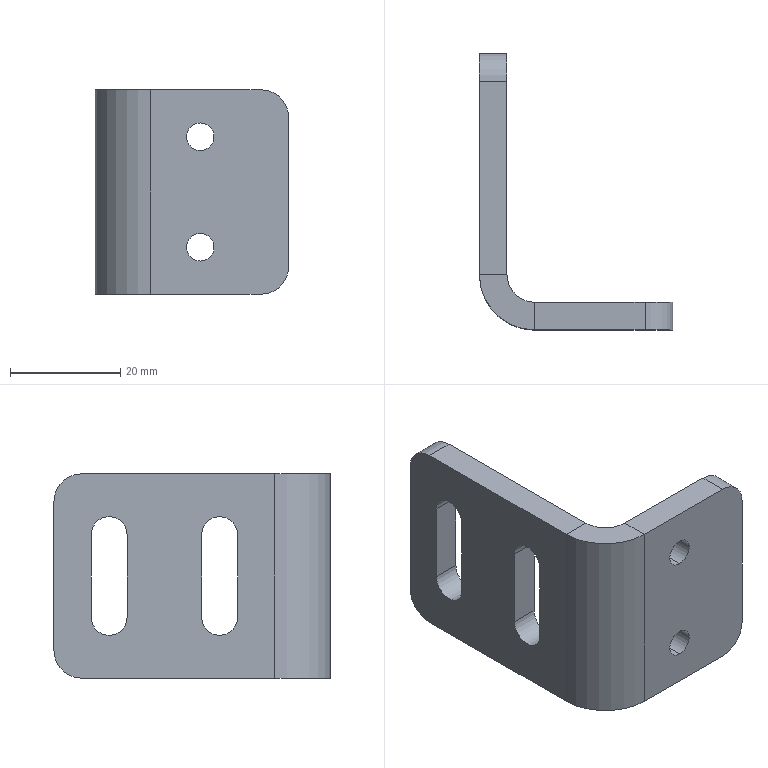Part | SolidWorks | features EdgeFlange 1, Fillet 1, FlatPattern 1, HoleWzd 1, ICE 1, SMBaseFlange 1, SheetMetal 1 | 1 solid | 30 faces | box 35 x 50 x 37 mm | volume 12594 mm3 | plane 16 | cylinder 14 | commonest cylinder face diameters 10 x5 5 x4 6.5 x4 20 x1
STEP:
#1=CARTESIAN_POINT('',(1.5,-5.,-12.5));
#2=VERTEX_POINT('',#1);
#3=CARTESIAN_POINT('',(1.5,-5.,-7.5));
#4=VERTEX_POINT('',#3);
#5=CARTESIAN_POINT('',(1.5,-5.,-10.));
#6=DIRECTION('',(0.,1.,0.));
#7=DIRECTION('',(0.,0.,1.));
#8=AXIS2_PLACEMENT_3D('',#5,#6,#7);
#9=CIRCLE('',#8,2.5);
#10=EDGE_CURVE('',#2,#4,#9,.T.);
#11=ORIENTED_EDGE('',*,*,#10,.F.);
#12=CARTESIAN_POINT('',(1.5,0.,-12.5));
#13=VERTEX_POINT('',#12);
#14=CARTESIAN_POINT('',(1.5,0.,-12.5));
#15=DIRECTION('',(0.,1.,0.));
#16=VECTOR('',#15,1000.);
#17=LINE('',#14,#16);
#18=EDGE_CURVE('',#2,#13,#17,.T.);
#19=ORIENTED_EDGE('',*,*,#18,.T.);
#20=CARTESIAN_POINT('',(1.5,0.,-7.5));
#21=VERTEX_POINT('',#20);
#22=CARTESIAN_POINT('',(1.5,0.,-10.));
#23=DIRECTION('',(0.,1.,0.));
#24=DIRECTION('',(0.,0.,1.));
#25=AXIS2_PLACEMENT_3D('',#22,#23,#24);
#26=CIRCLE('',#25,2.5);
#27=EDGE_CURVE('',#13,#21,#26,.T.);
#28=ORIENTED_EDGE('',*,*,#27,.T.);
#29=CARTESIAN_POINT('',(1.5,0.,-7.5));
#30=DIRECTION('',(0.,1.,0.));
#31=VECTOR('',#30,1000.);
#32=LINE('',#29,#31);
#33=EDGE_CURVE('',#4,#21,#32,.T.);
#34=ORIENTED_EDGE('',*,*,#33,.F.);
#35=EDGE_LOOP('',(#11,#19,#28,#34));
#36=FACE_OUTER_BOUND('',#35,.T.);
#37=CARTESIAN_POINT('',(1.5,0.,-10.));
#38=DIRECTION('',(0.,1.,0.));
#39=DIRECTION('',(0.,0.,1.));
#40=AXIS2_PLACEMENT_3D('',#37,#38,#39);
#41=CYLINDRICAL_SURFACE('',#40,2.5);
#42=ADVANCED_FACE('',(#36),#41,.F.);
#43=CARTESIAN_POINT('',(1.5,-5.,7.5));
#44=VERTEX_POINT('',#43);
#45=CARTESIAN_POINT('',(1.5,-5.,12.5));
#46=VERTEX_POINT('',#45);
#47=CARTESIAN_POINT('',(1.5,-5.,10.));
#48=DIRECTION('',(0.,1.,0.));
#49=DIRECTION('',(0.,0.,1.));
#50=AXIS2_PLACEMENT_3D('',#47,#48,#49);
#51=CIRCLE('',#50,2.5);
#52=EDGE_CURVE('',#44,#46,#51,.T.);
#53=ORIENTED_EDGE('',*,*,#52,.F.);
#54=CARTESIAN_POINT('',(1.5,0.,7.5));
#55=VERTEX_POINT('',#54);
#56=CARTESIAN_POINT('',(1.5,0.,7.5));
#57=DIRECTION('',(0.,1.,0.));
#58=VECTOR('',#57,1000.);
#59=LINE('',#56,#58);
#60=EDGE_CURVE('',#44,#55,#59,.T.);
#61=ORIENTED_EDGE('',*,*,#60,.T.);
#62=CARTESIAN_POINT('',(1.5,0.,12.5));
#63=VERTEX_POINT('',#62);
#64=CARTESIAN_POINT('',(1.5,0.,10.));
#65=DIRECTION('',(0.,1.,0.));
#66=DIRECTION('',(0.,0.,1.));
#67=AXIS2_PLACEMENT_3D('',#64,#65,#66);
#68=CIRCLE('',#67,2.5);
#69=EDGE_CURVE('',#55,#63,#68,.T.);
#70=ORIENTED_EDGE('',*,*,#69,.T.);
#71=CARTESIAN_POINT('',(1.5,0.,12.5));
#72=DIRECTION('',(0.,1.,0.));
#73=VECTOR('',#72,1000.);
#74=LINE('',#71,#73);
#75=EDGE_CURVE('',#46,#63,#74,.T.);
#76=ORIENTED_EDGE('',*,*,#75,.F.);
#77=EDGE_LOOP('',(#53,#61,#70,#76));
#78=FACE_OUTER_BOUND('',#77,.T.);
#79=CARTESIAN_POINT('',(1.5,0.,10.));
#80=DIRECTION('',(0.,1.,0.));
#81=DIRECTION('',(0.,0.,1.));
#82=AXIS2_PLACEMENT_3D('',#79,#80,#81);
#83=CYLINDRICAL_SURFACE('',#82,2.5);
#84=ADVANCED_FACE('',(#78),#83,.F.);
#85=CARTESIAN_POINT('',(-7.5,-5.,18.5));
#86=VERTEX_POINT('',#85);
#87=CARTESIAN_POINT('',(12.5,-5.,18.5));
#88=VERTEX_POINT('',#87);
#89=CARTESIAN_POINT('',(17.5,-5.,18.5));
#90=DIRECTION('',(1.,0.,0.));
#91=VECTOR('',#90,1000.);
#92=LINE('',#89,#91);
#93=EDGE_CURVE('',#86,#88,#92,.T.);
#94=ORIENTED_EDGE('',*,*,#93,.T.);
#95=CARTESIAN_POINT('',(12.5,0.,18.5));
#96=VERTEX_POINT('',#95);
#97=CARTESIAN_POINT('',(12.5,-5.,18.5));
#98=DIRECTION('',(0.,1.,0.));
#99=VECTOR('',#98,1000.);
#100=LINE('',#97,#99);
#101=EDGE_CURVE('',#88,#96,#100,.T.);
#102=ORIENTED_EDGE('',*,*,#101,.T.);
#103=CARTESIAN_POINT('',(-7.5,0.,18.5));
#104=VERTEX_POINT('',#103);
#105=CARTESIAN_POINT('',(17.5,0.,18.5));
#106=DIRECTION('',(1.,0.,0.));
#107=VECTOR('',#106,1000.);
#108=LINE('',#105,#107);
#109=EDGE_CURVE('',#104,#96,#108,.T.);
#110=ORIENTED_EDGE('',*,*,#109,.F.);
#111=CARTESIAN_POINT('',(-7.5,0.,18.5));
#112=DIRECTION('',(0.,-1.,0.));
#113=VECTOR('',#112,1000.);
#114=LINE('',#111,#113);
#115=EDGE_CURVE('',#104,#86,#114,.T.);
#116=ORIENTED_EDGE('',*,*,#115,.T.);
#117=EDGE_LOOP('',(#94,#102,#110,#116));
#118=FACE_OUTER_BOUND('',#117,.T.);
#119=CARTESIAN_POINT('',(17.5,-5.,18.5));
#120=DIRECTION('',(0.,0.,1.));
#121=DIRECTION('',(1.,0.,0.));
#122=AXIS2_PLACEMENT_3D('',#119,#120,#121);
#123=PLANE('',#122);
#124=ADVANCED_FACE('',(#118),#123,.T.);
#125=CARTESIAN_POINT('',(1.5,-5.,10.));
#126=DIRECTION('',(0.,1.,0.));
#127=DIRECTION('',(0.,0.,1.));
#128=AXIS2_PLACEMENT_3D('',#125,#126,#127);
#129=CIRCLE('',#128,2.5);
#130=EDGE_CURVE('',#46,#44,#129,.T.);
#131=ORIENTED_EDGE('',*,*,#130,.T.);
#132=ORIENTED_EDGE('',*,*,#52,.T.);
#133=EDGE_LOOP('',(#131,#132));
#134=FACE_BOUND('',#133,.T.);
#135=CARTESIAN_POINT('',(1.5,-5.,-10.));
#136=DIRECTION('',(0.,1.,0.));
#137=DIRECTION('',(0.,0.,1.));
#138=AXIS2_PLACEMENT_3D('',#135,#136,#137);
#139=CIRCLE('',#138,2.5);
#140=EDGE_CURVE('',#4,#2,#139,.T.);
#141=ORIENTED_EDGE('',*,*,#140,.T.);
#142=ORIENTED_EDGE('',*,*,#10,.T.);
#143=EDGE_LOOP('',(#141,#142));
#144=FACE_BOUND('',#143,.T.);
#145=CARTESIAN_POINT('',(17.5,-5.,13.5));
#146=VERTEX_POINT('',#145);
#147=CARTESIAN_POINT('',(17.5,-5.,-13.5));
#148=VERTEX_POINT('',#147);
#149=CARTESIAN_POINT('',(17.5,-5.,18.5));
#150=DIRECTION('',(0.,0.,-1.));
#151=VECTOR('',#150,1000.);
#152=LINE('',#149,#151);
#153=EDGE_CURVE('',#146,#148,#152,.T.);
#154=ORIENTED_EDGE('',*,*,#153,.F.);
#155=CARTESIAN_POINT('',(12.5,-5.,13.5));
#156=DIRECTION('',(0.,-1.,0.));
#157=DIRECTION('',(0.,0.,1.));
#158=AXIS2_PLACEMENT_3D('',#155,#156,#157);
#159=CIRCLE('',#158,5.);
#160=EDGE_CURVE('',#146,#88,#159,.T.);
#161=ORIENTED_EDGE('',*,*,#160,.T.);
#162=ORIENTED_EDGE('',*,*,#93,.F.);
#163=CARTESIAN_POINT('',(-7.5,-5.,-18.5));
#164=VERTEX_POINT('',#163);
#165=CARTESIAN_POINT('',(-7.5,-5.,18.5));
#166=DIRECTION('',(0.,0.,-1.));
#167=VECTOR('',#166,1000.);
#168=LINE('',#165,#167);
#169=EDGE_CURVE('',#86,#164,#168,.T.);
#170=ORIENTED_EDGE('',*,*,#169,.T.);
#171=CARTESIAN_POINT('',(12.5,-5.,-18.5));
#172=VERTEX_POINT('',#171);
#173=CARTESIAN_POINT('',(17.5,-5.,-18.5));
#174=DIRECTION('',(-1.,0.,0.));
#175=VECTOR('',#174,1000.);
#176=LINE('',#173,#175);
#177=EDGE_CURVE('',#172,#164,#176,.T.);
#178=ORIENTED_EDGE('',*,*,#177,.F.);
#179=CARTESIAN_POINT('',(12.5,-5.,-13.5));
#180=DIRECTION('',(0.,-1.,0.));
#181=DIRECTION('',(0.,0.,1.));
#182=AXIS2_PLACEMENT_3D('',#179,#180,#181);
#183=CIRCLE('',#182,5.);
#184=EDGE_CURVE('',#172,#148,#183,.T.);
#185=ORIENTED_EDGE('',*,*,#184,.T.);
#186=EDGE_LOOP('',(#154,#161,#162,#170,#178,#185));
#187=FACE_OUTER_BOUND('',#186,.T.);
#188=CARTESIAN_POINT('',(0.,-5.,0.));
#189=DIRECTION('',(0.,1.,0.));
#190=DIRECTION('',(0.,0.,1.));
#191=AXIS2_PLACEMENT_3D('',#188,#189,#190);
#192=PLANE('',#191);
#193=ADVANCED_FACE('',(#134,#144,#187),#192,.F.);
#194=CARTESIAN_POINT('',(1.5,0.,-10.));
#195=DIRECTION('',(0.,1.,0.));
#196=DIRECTION('',(0.,0.,1.));
#197=AXIS2_PLACEMENT_3D('',#194,#195,#196);
#198=CIRCLE('',#197,2.5);
#199=EDGE_CURVE('',#21,#13,#198,.T.);
#200=ORIENTED_EDGE('',*,*,#199,.F.);
#201=ORIENTED_EDGE('',*,*,#27,.F.);
#202=EDGE_LOOP('',(#200,#201));
#203=FACE_BOUND('',#202,.T.);
#204=CARTESIAN_POINT('',(1.5,0.,10.));
#205=DIRECTION('',(0.,1.,0.));
#206=DIRECTION('',(0.,0.,1.));
#207=AXIS2_PLACEMENT_3D('',#204,#205,#206);
#208=CIRCLE('',#207,2.5);
#209=EDGE_CURVE('',#63,#55,#208,.T.);
#210=ORIENTED_EDGE('',*,*,#209,.F.);
#211=ORIENTED_EDGE('',*,*,#69,.F.);
#212=EDGE_LOOP('',(#210,#211));
#213=FACE_BOUND('',#212,.T.);
#214=ORIENTED_EDGE('',*,*,#109,.T.);
#215=CARTESIAN_POINT('',(17.5,0.,13.5));
#216=VERTEX_POINT('',#215);
#217=CARTESIAN_POINT('',(12.5,0.,13.5));
#218=DIRECTION('',(0.,1.,0.));
#219=DIRECTION('',(0.,0.,1.));
#220=AXIS2_PLACEMENT_3D('',#217,#218,#219);
#221=CIRCLE('',#220,5.);
#222=EDGE_CURVE('',#96,#216,#221,.T.);
#223=ORIENTED_EDGE('',*,*,#222,.T.);
#224=CARTESIAN_POINT('',(17.5,0.,-13.5));
#225=VERTEX_POINT('',#224);
#226=CARTESIAN_POINT('',(17.5,0.,18.5));
#227=DIRECTION('',(0.,0.,-1.));
#228=VECTOR('',#227,1000.);
#229=LINE('',#226,#228);
#230=EDGE_CURVE('',#216,#225,#229,.T.);
#231=ORIENTED_EDGE('',*,*,#230,.T.);
#232=CARTESIAN_POINT('',(12.5,0.,-18.5));
#233=VERTEX_POINT('',#232);
#234=CARTESIAN_POINT('',(12.5,0.,-13.5));
#235=DIRECTION('',(0.,1.,0.));
#236=DIRECTION('',(0.,0.,1.));
#237=AXIS2_PLACEMENT_3D('',#234,#235,#236);
#238=CIRCLE('',#237,5.);
#239=EDGE_CURVE('',#225,#233,#238,.T.);
#240=ORIENTED_EDGE('',*,*,#239,.T.);
#241=CARTESIAN_POINT('',(-7.5,0.,-18.5));
#242=VERTEX_POINT('',#241);
#243=CARTESIAN_POINT('',(17.5,0.,-18.5));
#244=DIRECTION('',(-1.,0.,0.));
#245=VECTOR('',#244,1000.);
#246=LINE('',#243,#245);
#247=EDGE_CURVE('',#233,#242,#246,.T.);
#248=ORIENTED_EDGE('',*,*,#247,.T.);
#249=CARTESIAN_POINT('',(-7.5,0.,18.5));
#250=DIRECTION('',(0.,0.,-1.));
#251=VECTOR('',#250,1000.);
#252=LINE('',#249,#251);
#253=EDGE_CURVE('',#104,#242,#252,.T.);
#254=ORIENTED_EDGE('',*,*,#253,.F.);
#255=EDGE_LOOP('',(#214,#223,#231,#240,#248,#254));
#256=FACE_OUTER_BOUND('',#255,.T.);
#257=CARTESIAN_POINT('',(0.,0.,0.));
#258=DIRECTION('',(0.,1.,0.));
#259=DIRECTION('',(0.,0.,1.));
#260=AXIS2_PLACEMENT_3D('',#257,#258,#259);
#261=PLANE('',#260);
#262=ADVANCED_FACE('',(#203,#213,#256),#261,.T.);
#263=ORIENTED_EDGE('',*,*,#247,.F.);
#264=CARTESIAN_POINT('',(12.5,-5.,-18.5));
#265=DIRECTION('',(0.,-1.,0.));
#266=VECTOR('',#265,1000.);
#267=LINE('',#264,#266);
#268=EDGE_CURVE('',#233,#172,#267,.T.);
#269=ORIENTED_EDGE('',*,*,#268,.T.);
#270=ORIENTED_EDGE('',*,*,#177,.T.);
#271=CARTESIAN_POINT('',(-7.5,0.,-18.5));
#272=DIRECTION('',(0.,-1.,0.));
#273=VECTOR('',#272,1000.);
#274=LINE('',#271,#273);
#275=EDGE_CURVE('',#242,#164,#274,.T.);
#276=ORIENTED_EDGE('',*,*,#275,.F.);
#277=EDGE_LOOP('',(#263,#269,#270,#276));
#278=FACE_OUTER_BOUND('',#277,.T.);
#279=CARTESIAN_POINT('',(17.5,-5.,-18.5));
#280=DIRECTION('',(0.,0.,-1.));
#281=DIRECTION('',(-1.,0.,0.));
#282=AXIS2_PLACEMENT_3D('',#279,#280,#281);
#283=PLANE('',#282);
#284=ADVANCED_FACE('',(#278),#283,.T.);
#285=ORIENTED_EDGE('',*,*,#230,.F.);
#286=CARTESIAN_POINT('',(17.5,-5.,13.5));
#287=DIRECTION('',(0.,-1.,0.));
#288=VECTOR('',#287,1000.);
#289=LINE('',#286,#288);
#290=EDGE_CURVE('',#216,#146,#289,.T.);
#291=ORIENTED_EDGE('',*,*,#290,.T.);
#292=ORIENTED_EDGE('',*,*,#153,.T.);
#293=CARTESIAN_POINT('',(17.5,-5.,-13.5));
#294=DIRECTION('',(0.,1.,0.));
#295=VECTOR('',#294,1000.);
#296=LINE('',#293,#295);
#297=EDGE_CURVE('',#148,#225,#296,.T.);
#298=ORIENTED_EDGE('',*,*,#297,.T.);
#299=EDGE_LOOP('',(#285,#291,#292,#298));
#300=FACE_OUTER_BOUND('',#299,.T.);
#301=CARTESIAN_POINT('',(17.5,-5.,18.5));
#302=DIRECTION('',(1.,0.,0.));
#303=DIRECTION('',(0.,0.,-1.));
#304=AXIS2_PLACEMENT_3D('',#301,#302,#303);
#305=PLANE('',#304);
#306=ADVANCED_FACE('',(#300),#305,.T.);
#307=ORIENTED_EDGE('',*,*,#60,.F.);
#308=ORIENTED_EDGE('',*,*,#130,.F.);
#309=ORIENTED_EDGE('',*,*,#75,.T.);
#310=ORIENTED_EDGE('',*,*,#209,.T.);
#311=EDGE_LOOP('',(#307,#308,#309,#310));
#312=FACE_OUTER_BOUND('',#311,.T.);
#313=CARTESIAN_POINT('',(1.5,0.,10.));
#314=DIRECTION('',(0.,1.,0.));
#315=DIRECTION('',(0.,0.,1.));
#316=AXIS2_PLACEMENT_3D('',#313,#314,#315);
#317=CYLINDRICAL_SURFACE('',#316,2.5);
#318=ADVANCED_FACE('',(#312),#317,.F.);
#319=ORIENTED_EDGE('',*,*,#18,.F.);
#320=ORIENTED_EDGE('',*,*,#140,.F.);
#321=ORIENTED_EDGE('',*,*,#33,.T.);
#322=ORIENTED_EDGE('',*,*,#199,.T.);
#323=EDGE_LOOP('',(#319,#320,#321,#322));
#324=FACE_OUTER_BOUND('',#323,.T.);
#325=CARTESIAN_POINT('',(1.5,0.,-10.));
#326=DIRECTION('',(0.,1.,0.));
#327=DIRECTION('',(0.,0.,1.));
#328=AXIS2_PLACEMENT_3D('',#325,#326,#327);
#329=CYLINDRICAL_SURFACE('',#328,2.5);
#330=ADVANCED_FACE('',(#324),#329,.F.);
#331=CARTESIAN_POINT('',(-12.5,5.,-18.5));
#332=VERTEX_POINT('',#331);
#333=CARTESIAN_POINT('',(-17.5,5.,-18.5));
#334=VERTEX_POINT('',#333);
#335=CARTESIAN_POINT('',(-17.5,5.,-18.5));
#336=DIRECTION('',(-1.,0.,0.));
#337=VECTOR('',#336,1000.);
#338=LINE('',#335,#337);
#339=EDGE_CURVE('',#332,#334,#338,.T.);
#340=ORIENTED_EDGE('',*,*,#339,.F.);
#341=CARTESIAN_POINT('',(-7.5,5.,-18.5));
#342=DIRECTION('',(0.,0.,-1.));
#343=DIRECTION('',(0.,-1.,0.));
#344=AXIS2_PLACEMENT_3D('',#341,#342,#343);
#345=CIRCLE('',#344,5.);
#346=EDGE_CURVE('',#242,#332,#345,.T.);
#347=ORIENTED_EDGE('',*,*,#346,.F.);
#348=ORIENTED_EDGE('',*,*,#275,.T.);
#349=CARTESIAN_POINT('',(-7.5,5.,-18.5));
#350=DIRECTION('',(0.,0.,-1.));
#351=DIRECTION('',(0.,-1.,0.));
#352=AXIS2_PLACEMENT_3D('',#349,#350,#351);
#353=CIRCLE('',#352,10.);
#354=EDGE_CURVE('',#164,#334,#353,.T.);
#355=ORIENTED_EDGE('',*,*,#354,.T.);
#356=EDGE_LOOP('',(#340,#347,#348,#355));
#357=FACE_OUTER_BOUND('',#356,.T.);
#358=CARTESIAN_POINT('',(-7.5,5.,-18.5));
#359=DIRECTION('',(0.,0.,-1.));
#360=DIRECTION('',(0.,1.,0.));
#361=AXIS2_PLACEMENT_3D('',#358,#359,#360);
#362=PLANE('',#361);
#363=ADVANCED_FACE('',(#357),#362,.T.);
#364=CARTESIAN_POINT('',(-12.5,5.,18.5));
#365=VERTEX_POINT('',#364);
#366=CARTESIAN_POINT('',(-7.5,5.,18.5));
#367=DIRECTION('',(0.,0.,1.));
#368=DIRECTION('',(0.,-1.,0.));
#369=AXIS2_PLACEMENT_3D('',#366,#367,#368);
#370=CIRCLE('',#369,5.);
#371=EDGE_CURVE('',#365,#104,#370,.T.);
#372=ORIENTED_EDGE('',*,*,#371,.F.);
#373=CARTESIAN_POINT('',(-17.5,5.,18.5));
#374=VERTEX_POINT('',#373);
#375=CARTESIAN_POINT('',(-12.5,5.,18.5));
#376=DIRECTION('',(-1.,0.,0.));
#377=VECTOR('',#376,1000.);
#378=LINE('',#375,#377);
#379=EDGE_CURVE('',#365,#374,#378,.T.);
#380=ORIENTED_EDGE('',*,*,#379,.T.);
#381=CARTESIAN_POINT('',(-7.5,5.,18.5));
#382=DIRECTION('',(0.,0.,1.));
#383=DIRECTION('',(0.,-1.,0.));
#384=AXIS2_PLACEMENT_3D('',#381,#382,#383);
#385=CIRCLE('',#384,10.);
#386=EDGE_CURVE('',#374,#86,#385,.T.);
#387=ORIENTED_EDGE('',*,*,#386,.T.);
#388=ORIENTED_EDGE('',*,*,#115,.F.);
#389=EDGE_LOOP('',(#372,#380,#387,#388));
#390=FACE_OUTER_BOUND('',#389,.T.);
#391=CARTESIAN_POINT('',(-7.5,5.,18.5));
#392=DIRECTION('',(0.,0.,-1.));
#393=DIRECTION('',(0.,1.,0.));
#394=AXIS2_PLACEMENT_3D('',#391,#392,#393);
#395=PLANE('',#394);
#396=ADVANCED_FACE('',(#390),#395,.F.);
#397=ORIENTED_EDGE('',*,*,#169,.F.);
#398=ORIENTED_EDGE('',*,*,#386,.F.);
#399=CARTESIAN_POINT('',(-17.5,5.,-18.5));
#400=DIRECTION('',(0.,0.,-1.));
#401=VECTOR('',#400,1000.);
#402=LINE('',#399,#401);
#403=EDGE_CURVE('',#374,#334,#402,.T.);
#404=ORIENTED_EDGE('',*,*,#403,.T.);
#405=ORIENTED_EDGE('',*,*,#354,.F.);
#406=EDGE_LOOP('',(#397,#398,#404,#405));
#407=FACE_OUTER_BOUND('',#406,.T.);
#408=CARTESIAN_POINT('',(-7.5,5.,18.5));
#409=DIRECTION('',(0.,0.,1.));
#410=DIRECTION('',(-1.,0.,0.));
#411=AXIS2_PLACEMENT_3D('',#408,#409,#410);
#412=CYLINDRICAL_SURFACE('',#411,10.);
#413=ADVANCED_FACE('',(#407),#412,.T.);
#414=ORIENTED_EDGE('',*,*,#253,.T.);
#415=ORIENTED_EDGE('',*,*,#346,.T.);
#416=CARTESIAN_POINT('',(-12.5,5.,-18.5));
#417=DIRECTION('',(0.,0.,1.));
#418=VECTOR('',#417,1000.);
#419=LINE('',#416,#418);
#420=EDGE_CURVE('',#332,#365,#419,.T.);
#421=ORIENTED_EDGE('',*,*,#420,.T.);
#422=ORIENTED_EDGE('',*,*,#371,.T.);
#423=EDGE_LOOP('',(#414,#415,#421,#422));
#424=FACE_OUTER_BOUND('',#423,.T.);
#425=CARTESIAN_POINT('',(-7.5,5.,18.5));
#426=DIRECTION('',(0.,0.,1.));
#427=DIRECTION('',(-1.,0.,0.));
#428=AXIS2_PLACEMENT_3D('',#425,#426,#427);
#429=CYLINDRICAL_SURFACE('',#428,5.);
#430=ADVANCED_FACE('',(#424),#429,.F.);
#431=CARTESIAN_POINT('',(-17.5,40.,-18.5));
#432=VERTEX_POINT('',#431);
#433=CARTESIAN_POINT('',(-17.5,0.,-18.5));
#434=DIRECTION('',(0.,-1.,0.));
#435=VECTOR('',#434,1000.);
#436=LINE('',#433,#435);
#437=EDGE_CURVE('',#432,#334,#436,.T.);
#438=ORIENTED_EDGE('',*,*,#437,.F.);
#439=CARTESIAN_POINT('',(-12.5,40.,-18.5));
#440=VERTEX_POINT('',#439);
#441=CARTESIAN_POINT('',(-17.5,40.,-18.5));
#442=DIRECTION('',(1.,0.,0.));
#443=VECTOR('',#442,1000.);
#444=LINE('',#441,#443);
#445=EDGE_CURVE('',#432,#440,#444,.T.);
#446=ORIENTED_EDGE('',*,*,#445,.T.);
#447=CARTESIAN_POINT('',(-12.5,0.,-18.5));
#448=DIRECTION('',(0.,-1.,0.));
#449=VECTOR('',#448,1000.);
#450=LINE('',#447,#449);
#451=EDGE_CURVE('',#440,#332,#450,.T.);
#452=ORIENTED_EDGE('',*,*,#451,.T.);
#453=ORIENTED_EDGE('',*,*,#339,.T.);
#454=EDGE_LOOP('',(#438,#446,#452,#453));
#455=FACE_OUTER_BOUND('',#454,.T.);
#456=CARTESIAN_POINT('',(-17.5,0.,-18.5));
#457=DIRECTION('',(0.,0.,1.));
#458=DIRECTION('',(1.,0.,0.));
#459=AXIS2_PLACEMENT_3D('',#456,#457,#458);
#460=PLANE('',#459);
#461=ADVANCED_FACE('',(#455),#460,.F.);
#462=CARTESIAN_POINT('',(-12.5,40.,18.5));
#463=VERTEX_POINT('',#462);
#464=CARTESIAN_POINT('',(-12.5,45.,18.5));
#465=DIRECTION('',(0.,1.,0.));
#466=VECTOR('',#465,1000.);
#467=LINE('',#464,#466);
#468=EDGE_CURVE('',#365,#463,#467,.T.);
#469=ORIENTED_EDGE('',*,*,#468,.T.);
#470=CARTESIAN_POINT('',(-17.5,40.,18.5));
#471=VERTEX_POINT('',#470);
#472=CARTESIAN_POINT('',(-17.5,40.,18.5));
#473=DIRECTION('',(-1.,0.,0.));
#474=VECTOR('',#473,1000.);
#475=LINE('',#472,#474);
#476=EDGE_CURVE('',#463,#471,#475,.T.);
#477=ORIENTED_EDGE('',*,*,#476,.T.);
#478=CARTESIAN_POINT('',(-17.5,0.,18.5));
#479=DIRECTION('',(0.,1.,0.));
#480=VECTOR('',#479,1000.);
#481=LINE('',#478,#480);
#482=EDGE_CURVE('',#374,#471,#481,.T.);
#483=ORIENTED_EDGE('',*,*,#482,.F.);
#484=ORIENTED_EDGE('',*,*,#379,.F.);
#485=EDGE_LOOP('',(#469,#477,#483,#484));
#486=FACE_OUTER_BOUND('',#485,.T.);
#487=CARTESIAN_POINT('',(-17.5,45.,18.5));
#488=DIRECTION('',(0.,0.,-1.));
#489=DIRECTION('',(-1.,0.,0.));
#490=AXIS2_PLACEMENT_3D('',#487,#488,#489);
#491=PLANE('',#490);
#492=ADVANCED_FACE('',(#486),#491,.F.);
#493=CARTESIAN_POINT('',(-17.5,31.75,7.5));
#494=VERTEX_POINT('',#493);
#495=CARTESIAN_POINT('',(-17.5,31.75,-7.5));
#496=VERTEX_POINT('',#495);
#497=CARTESIAN_POINT('',(-17.5,31.75,0.));
#498=DIRECTION('',(0.,0.,-1.));
#499=VECTOR('',#498,1000.);
#500=LINE('',#497,#499);
#501=EDGE_CURVE('',#494,#496,#500,.T.);
#502=ORIENTED_EDGE('',*,*,#501,.T.);
#503=CARTESIAN_POINT('',(-17.5,38.25,-7.5));
#504=VERTEX_POINT('',#503);
#505=CARTESIAN_POINT('',(-17.5,35.,-7.5));
#506=DIRECTION('',(1.,0.,0.));
#507=DIRECTION('',(0.,1.,0.));
#508=AXIS2_PLACEMENT_3D('',#505,#506,#507);
#509=CIRCLE('',#508,3.25);
#510=EDGE_CURVE('',#496,#504,#509,.T.);
#511=ORIENTED_EDGE('',*,*,#510,.T.);
#512=CARTESIAN_POINT('',(-17.5,38.25,7.5));
#513=VERTEX_POINT('',#512);
#514=CARTESIAN_POINT('',(-17.5,38.25,0.));
#515=DIRECTION('',(0.,0.,1.));
#516=VECTOR('',#515,1000.);
#517=LINE('',#514,#516);
#518=EDGE_CURVE('',#504,#513,#517,.T.);
#519=ORIENTED_EDGE('',*,*,#518,.T.);
#520=CARTESIAN_POINT('',(-17.5,35.,7.5));
#521=DIRECTION('',(1.,0.,0.));
#522=DIRECTION('',(0.,1.,0.));
#523=AXIS2_PLACEMENT_3D('',#520,#521,#522);
#524=CIRCLE('',#523,3.25);
#525=EDGE_CURVE('',#513,#494,#524,.T.);
#526=ORIENTED_EDGE('',*,*,#525,.T.);
#527=EDGE_LOOP('',(#502,#511,#519,#526));
#528=FACE_BOUND('',#527,.T.);
#529=CARTESIAN_POINT('',(-17.5,11.75,7.5));
#530=VERTEX_POINT('',#529);
#531=CARTESIAN_POINT('',(-17.5,11.75,-7.5));
#532=VERTEX_POINT('',#531);
#533=CARTESIAN_POINT('',(-17.5,11.75,0.));
#534=DIRECTION('',(0.,0.,-1.));
#535=VECTOR('',#534,1000.);
#536=LINE('',#533,#535);
#537=EDGE_CURVE('',#530,#532,#536,.T.);
#538=ORIENTED_EDGE('',*,*,#537,.T.);
#539=CARTESIAN_POINT('',(-17.5,18.25,-7.5));
#540=VERTEX_POINT('',#539);
#541=CARTESIAN_POINT('',(-17.5,15.,-7.5));
#542=DIRECTION('',(1.,0.,0.));
#543=DIRECTION('',(0.,1.,0.));
#544=AXIS2_PLACEMENT_3D('',#541,#542,#543);
#545=CIRCLE('',#544,3.25);
#546=EDGE_CURVE('',#532,#540,#545,.T.);
#547=ORIENTED_EDGE('',*,*,#546,.T.);
#548=CARTESIAN_POINT('',(-17.5,18.25,7.5));
#549=VERTEX_POINT('',#548);
#550=CARTESIAN_POINT('',(-17.5,18.25,0.));
#551=DIRECTION('',(0.,0.,1.));
#552=VECTOR('',#551,1000.);
#553=LINE('',#550,#552);
#554=EDGE_CURVE('',#540,#549,#553,.T.);
#555=ORIENTED_EDGE('',*,*,#554,.T.);
#556=CARTESIAN_POINT('',(-17.5,15.,7.5));
#557=DIRECTION('',(1.,0.,0.));
#558=DIRECTION('',(0.,1.,0.));
#559=AXIS2_PLACEMENT_3D('',#556,#557,#558);
#560=CIRCLE('',#559,3.25);
#561=EDGE_CURVE('',#549,#530,#560,.T.);
#562=ORIENTED_EDGE('',*,*,#561,.T.);
#563=EDGE_LOOP('',(#538,#547,#555,#562));
#564=FACE_BOUND('',#563,.T.);
#565=CARTESIAN_POINT('',(-17.5,45.,13.5));
#566=VERTEX_POINT('',#565);
#567=CARTESIAN_POINT('',(-17.5,45.,-13.5));
#568=VERTEX_POINT('',#567);
#569=CARTESIAN_POINT('',(-17.5,45.,0.));
#570=DIRECTION('',(0.,0.,-1.));
#571=VECTOR('',#570,1000.);
#572=LINE('',#569,#571);
#573=EDGE_CURVE('',#566,#568,#572,.T.);
#574=ORIENTED_EDGE('',*,*,#573,.T.);
#575=CARTESIAN_POINT('',(-17.5,40.,-13.5));
#576=DIRECTION('',(-1.,0.,0.));
#577=DIRECTION('',(0.,1.,0.));
#578=AXIS2_PLACEMENT_3D('',#575,#576,#577);
#579=CIRCLE('',#578,5.);
#580=EDGE_CURVE('',#568,#432,#579,.T.);
#581=ORIENTED_EDGE('',*,*,#580,.T.);
#582=ORIENTED_EDGE('',*,*,#437,.T.);
#583=ORIENTED_EDGE('',*,*,#403,.F.);
#584=ORIENTED_EDGE('',*,*,#482,.T.);
#585=CARTESIAN_POINT('',(-17.5,40.,13.5));
#586=DIRECTION('',(-1.,0.,0.));
#587=DIRECTION('',(0.,1.,0.));
#588=AXIS2_PLACEMENT_3D('',#585,#586,#587);
#589=CIRCLE('',#588,5.);
#590=EDGE_CURVE('',#471,#566,#589,.T.);
#591=ORIENTED_EDGE('',*,*,#590,.T.);
#592=EDGE_LOOP('',(#574,#581,#582,#583,#584,#591));
#593=FACE_OUTER_BOUND('',#592,.T.);
#594=CARTESIAN_POINT('',(-17.5,0.,0.));
#595=DIRECTION('',(1.,0.,0.));
#596=DIRECTION('',(0.,1.,0.));
#597=AXIS2_PLACEMENT_3D('',#594,#595,#596);
#598=PLANE('',#597);
#599=ADVANCED_FACE('',(#528,#564,#593),#598,.F.);
#600=CARTESIAN_POINT('',(-12.5,31.75,-7.5));
#601=VERTEX_POINT('',#600);
#602=CARTESIAN_POINT('',(-12.5,38.25,-7.5));
#603=VERTEX_POINT('',#602);
#604=CARTESIAN_POINT('',(-12.5,35.,-7.5));
#605=DIRECTION('',(1.,0.,0.));
#606=DIRECTION('',(0.,1.,0.));
#607=AXIS2_PLACEMENT_3D('',#604,#605,#606);
#608=CIRCLE('',#607,3.25);
#609=EDGE_CURVE('',#601,#603,#608,.T.);
#610=ORIENTED_EDGE('',*,*,#609,.F.);
#611=CARTESIAN_POINT('',(-12.5,31.75,7.5));
#612=VERTEX_POINT('',#611);
#613=CARTESIAN_POINT('',(-12.5,31.75,-7.5));
#614=DIRECTION('',(0.,0.,-1.));
#615=VECTOR('',#614,1000.);
#616=LINE('',#613,#615);
#617=EDGE_CURVE('',#612,#601,#616,.T.);
#618=ORIENTED_EDGE('',*,*,#617,.F.);
#619=CARTESIAN_POINT('',(-12.5,38.25,7.5));
#620=VERTEX_POINT('',#619);
#621=CARTESIAN_POINT('',(-12.5,35.,7.5));
#622=DIRECTION('',(1.,0.,0.));
#623=DIRECTION('',(0.,1.,0.));
#624=AXIS2_PLACEMENT_3D('',#621,#622,#623);
#625=CIRCLE('',#624,3.25);
#626=EDGE_CURVE('',#620,#612,#625,.T.);
#627=ORIENTED_EDGE('',*,*,#626,.F.);
#628=CARTESIAN_POINT('',(-12.5,38.25,-7.5));
#629=DIRECTION('',(0.,0.,1.));
#630=VECTOR('',#629,1000.);
#631=LINE('',#628,#630);
#632=EDGE_CURVE('',#603,#620,#631,.T.);
#633=ORIENTED_EDGE('',*,*,#632,.F.);
#634=EDGE_LOOP('',(#610,#618,#627,#633));
#635=FACE_BOUND('',#634,.T.);
#636=CARTESIAN_POINT('',(-12.5,11.75,-7.5));
#637=VERTEX_POINT('',#636);
#638=CARTESIAN_POINT('',(-12.5,18.25,-7.5));
#639=VERTEX_POINT('',#638);
#640=CARTESIAN_POINT('',(-12.5,15.,-7.5));
#641=DIRECTION('',(1.,0.,0.));
#642=DIRECTION('',(0.,1.,0.));
#643=AXIS2_PLACEMENT_3D('',#640,#641,#642);
#644=CIRCLE('',#643,3.25);
#645=EDGE_CURVE('',#637,#639,#644,.T.);
#646=ORIENTED_EDGE('',*,*,#645,.F.);
#647=CARTESIAN_POINT('',(-12.5,11.75,7.5));
#648=VERTEX_POINT('',#647);
#649=CARTESIAN_POINT('',(-12.5,11.75,-7.5));
#650=DIRECTION('',(0.,0.,-1.));
#651=VECTOR('',#650,1000.);
#652=LINE('',#649,#651);
#653=EDGE_CURVE('',#648,#637,#652,.T.);
#654=ORIENTED_EDGE('',*,*,#653,.F.);
#655=CARTESIAN_POINT('',(-12.5,18.25,7.5));
#656=VERTEX_POINT('',#655);
#657=CARTESIAN_POINT('',(-12.5,15.,7.5));
#658=DIRECTION('',(1.,0.,0.));
#659=DIRECTION('',(0.,1.,0.));
#660=AXIS2_PLACEMENT_3D('',#657,#658,#659);
#661=CIRCLE('',#660,3.25);
#662=EDGE_CURVE('',#656,#648,#661,.T.);
#663=ORIENTED_EDGE('',*,*,#662,.F.);
#664=CARTESIAN_POINT('',(-12.5,18.25,-7.5));
#665=DIRECTION('',(0.,0.,1.));
#666=VECTOR('',#665,1000.);
#667=LINE('',#664,#666);
#668=EDGE_CURVE('',#639,#656,#667,.T.);
#669=ORIENTED_EDGE('',*,*,#668,.F.);
#670=EDGE_LOOP('',(#646,#654,#663,#669));
#671=FACE_BOUND('',#670,.T.);
#672=ORIENTED_EDGE('',*,*,#451,.F.);
#673=CARTESIAN_POINT('',(-12.5,45.,-13.5));
#674=VERTEX_POINT('',#673);
#675=CARTESIAN_POINT('',(-12.5,40.,-13.5));
#676=DIRECTION('',(1.,0.,0.));
#677=DIRECTION('',(0.,1.,0.));
#678=AXIS2_PLACEMENT_3D('',#675,#676,#677);
#679=CIRCLE('',#678,5.);
#680=EDGE_CURVE('',#440,#674,#679,.T.);
#681=ORIENTED_EDGE('',*,*,#680,.T.);
#682=CARTESIAN_POINT('',(-12.5,45.,13.5));
#683=VERTEX_POINT('',#682);
#684=CARTESIAN_POINT('',(-12.5,45.,-18.5));
#685=DIRECTION('',(0.,0.,-1.));
#686=VECTOR('',#685,1000.);
#687=LINE('',#684,#686);
#688=EDGE_CURVE('',#683,#674,#687,.T.);
#689=ORIENTED_EDGE('',*,*,#688,.F.);
#690=CARTESIAN_POINT('',(-12.5,40.,13.5));
#691=DIRECTION('',(1.,0.,0.));
#692=DIRECTION('',(0.,1.,0.));
#693=AXIS2_PLACEMENT_3D('',#690,#691,#692);
#694=CIRCLE('',#693,5.);
#695=EDGE_CURVE('',#683,#463,#694,.T.);
#696=ORIENTED_EDGE('',*,*,#695,.T.);
#697=ORIENTED_EDGE('',*,*,#468,.F.);
#698=ORIENTED_EDGE('',*,*,#420,.F.);
#699=EDGE_LOOP('',(#672,#681,#689,#696,#697,#698));
#700=FACE_OUTER_BOUND('',#699,.T.);
#701=CARTESIAN_POINT('',(-12.5,0.,0.));
#702=DIRECTION('',(1.,0.,0.));
#703=DIRECTION('',(0.,1.,0.));
#704=AXIS2_PLACEMENT_3D('',#701,#702,#703);
#705=PLANE('',#704);
#706=ADVANCED_FACE('',(#635,#671,#700),#705,.T.);
#707=ORIENTED_EDGE('',*,*,#688,.T.);
#708=CARTESIAN_POINT('',(-17.5,45.,-13.5));
#709=DIRECTION('',(-1.,0.,0.));
#710=VECTOR('',#709,1000.);
#711=LINE('',#708,#710);
#712=EDGE_CURVE('',#674,#568,#711,.T.);
#713=ORIENTED_EDGE('',*,*,#712,.T.);
#714=ORIENTED_EDGE('',*,*,#573,.F.);
#715=CARTESIAN_POINT('',(-17.5,45.,13.5));
#716=DIRECTION('',(1.,0.,0.));
#717=VECTOR('',#716,1000.);
#718=LINE('',#715,#717);
#719=EDGE_CURVE('',#566,#683,#718,.T.);
#720=ORIENTED_EDGE('',*,*,#719,.T.);
#721=EDGE_LOOP('',(#707,#713,#714,#720));
#722=FACE_OUTER_BOUND('',#721,.T.);
#723=CARTESIAN_POINT('',(-17.5,45.,-18.5));
#724=DIRECTION('',(0.,-1.,0.));
#725=DIRECTION('',(1.,0.,0.));
#726=AXIS2_PLACEMENT_3D('',#723,#724,#725);
#727=PLANE('',#726);
#728=ADVANCED_FACE('',(#722),#727,.F.);
#729=CARTESIAN_POINT('',(-22.5,11.75,-7.5));
#730=DIRECTION('',(1.,0.,0.));
#731=VECTOR('',#730,1000.);
#732=LINE('',#729,#731);
#733=EDGE_CURVE('',#532,#637,#732,.T.);
#734=ORIENTED_EDGE('',*,*,#733,.T.);
#735=ORIENTED_EDGE('',*,*,#645,.T.);
#736=CARTESIAN_POINT('',(-22.5,18.25,-7.5));
#737=DIRECTION('',(1.,0.,0.));
#738=VECTOR('',#737,1000.);
#739=LINE('',#736,#738);
#740=EDGE_CURVE('',#540,#639,#739,.T.);
#741=ORIENTED_EDGE('',*,*,#740,.F.);
#742=ORIENTED_EDGE('',*,*,#546,.F.);
#743=EDGE_LOOP('',(#734,#735,#741,#742));
#744=FACE_OUTER_BOUND('',#743,.T.);
#745=CARTESIAN_POINT('',(-22.5,15.,-7.5));
#746=DIRECTION('',(1.,0.,0.));
#747=DIRECTION('',(0.,1.,0.));
#748=AXIS2_PLACEMENT_3D('',#745,#746,#747);
#749=CYLINDRICAL_SURFACE('',#748,3.25);
#750=ADVANCED_FACE('',(#744),#749,.F.);
#751=CARTESIAN_POINT('',(-22.5,11.75,7.5));
#752=DIRECTION('',(1.,0.,0.));
#753=VECTOR('',#752,1000.);
#754=LINE('',#751,#753);
#755=EDGE_CURVE('',#530,#648,#754,.T.);
#756=ORIENTED_EDGE('',*,*,#755,.T.);
#757=ORIENTED_EDGE('',*,*,#653,.T.);
#758=ORIENTED_EDGE('',*,*,#733,.F.);
#759=ORIENTED_EDGE('',*,*,#537,.F.);
#760=EDGE_LOOP('',(#756,#757,#758,#759));
#761=FACE_OUTER_BOUND('',#760,.T.);
#762=CARTESIAN_POINT('',(-22.5,11.75,-7.5));
#763=DIRECTION('',(0.,-1.,0.));
#764=DIRECTION('',(1.,0.,0.));
#765=AXIS2_PLACEMENT_3D('',#762,#763,#764);
#766=PLANE('',#765);
#767=ADVANCED_FACE('',(#761),#766,.F.);
#768=CARTESIAN_POINT('',(-22.5,18.25,7.5));
#769=DIRECTION('',(1.,0.,0.));
#770=VECTOR('',#769,1000.);
#771=LINE('',#768,#770);
#772=EDGE_CURVE('',#549,#656,#771,.T.);
#773=ORIENTED_EDGE('',*,*,#772,.T.);
#774=ORIENTED_EDGE('',*,*,#662,.T.);
#775=ORIENTED_EDGE('',*,*,#755,.F.);
#776=ORIENTED_EDGE('',*,*,#561,.F.);
#777=EDGE_LOOP('',(#773,#774,#775,#776));
#778=FACE_OUTER_BOUND('',#777,.T.);
#779=CARTESIAN_POINT('',(-22.5,15.,7.5));
#780=DIRECTION('',(1.,0.,0.));
#781=DIRECTION('',(0.,1.,0.));
#782=AXIS2_PLACEMENT_3D('',#779,#780,#781);
#783=CYLINDRICAL_SURFACE('',#782,3.25);
#784=ADVANCED_FACE('',(#778),#783,.F.);
#785=ORIENTED_EDGE('',*,*,#740,.T.);
#786=ORIENTED_EDGE('',*,*,#668,.T.);
#787=ORIENTED_EDGE('',*,*,#772,.F.);
#788=ORIENTED_EDGE('',*,*,#554,.F.);
#789=EDGE_LOOP('',(#785,#786,#787,#788));
#790=FACE_OUTER_BOUND('',#789,.T.);
#791=CARTESIAN_POINT('',(-22.5,18.25,-7.5));
#792=DIRECTION('',(0.,1.,0.));
#793=DIRECTION('',(-1.,0.,0.));
#794=AXIS2_PLACEMENT_3D('',#791,#792,#793);
#795=PLANE('',#794);
#796=ADVANCED_FACE('',(#790),#795,.F.);
#797=CARTESIAN_POINT('',(-22.5,31.75,-7.5));
#798=DIRECTION('',(1.,0.,0.));
#799=VECTOR('',#798,1000.);
#800=LINE('',#797,#799);
#801=EDGE_CURVE('',#496,#601,#800,.T.);
#802=ORIENTED_EDGE('',*,*,#801,.T.);
#803=ORIENTED_EDGE('',*,*,#609,.T.);
#804=CARTESIAN_POINT('',(-22.5,38.25,-7.5));
#805=DIRECTION('',(1.,0.,0.));
#806=VECTOR('',#805,1000.);
#807=LINE('',#804,#806);
#808=EDGE_CURVE('',#504,#603,#807,.T.);
#809=ORIENTED_EDGE('',*,*,#808,.F.);
#810=ORIENTED_EDGE('',*,*,#510,.F.);
#811=EDGE_LOOP('',(#802,#803,#809,#810));
#812=FACE_OUTER_BOUND('',#811,.T.);
#813=CARTESIAN_POINT('',(-22.5,35.,-7.5));
#814=DIRECTION('',(1.,0.,0.));
#815=DIRECTION('',(0.,1.,0.));
#816=AXIS2_PLACEMENT_3D('',#813,#814,#815);
#817=CYLINDRICAL_SURFACE('',#816,3.25);
#818=ADVANCED_FACE('',(#812),#817,.F.);
#819=CARTESIAN_POINT('',(-22.5,31.75,7.5));
#820=DIRECTION('',(1.,0.,0.));
#821=VECTOR('',#820,1000.);
#822=LINE('',#819,#821);
#823=EDGE_CURVE('',#494,#612,#822,.T.);
#824=ORIENTED_EDGE('',*,*,#823,.T.);
#825=ORIENTED_EDGE('',*,*,#617,.T.);
#826=ORIENTED_EDGE('',*,*,#801,.F.);
#827=ORIENTED_EDGE('',*,*,#501,.F.);
#828=EDGE_LOOP('',(#824,#825,#826,#827));
#829=FACE_OUTER_BOUND('',#828,.T.);
#830=CARTESIAN_POINT('',(-22.5,31.75,-7.5));
#831=DIRECTION('',(0.,-1.,0.));
#832=DIRECTION('',(1.,0.,0.));
#833=AXIS2_PLACEMENT_3D('',#830,#831,#832);
#834=PLANE('',#833);
#835=ADVANCED_FACE('',(#829),#834,.F.);
#836=CARTESIAN_POINT('',(-22.5,38.25,7.5));
#837=DIRECTION('',(1.,0.,0.));
#838=VECTOR('',#837,1000.);
#839=LINE('',#836,#838);
#840=EDGE_CURVE('',#513,#620,#839,.T.);
#841=ORIENTED_EDGE('',*,*,#840,.T.);
#842=ORIENTED_EDGE('',*,*,#626,.T.);
#843=ORIENTED_EDGE('',*,*,#823,.F.);
#844=ORIENTED_EDGE('',*,*,#525,.F.);
#845=EDGE_LOOP('',(#841,#842,#843,#844));
#846=FACE_OUTER_BOUND('',#845,.T.);
#847=CARTESIAN_POINT('',(-22.5,35.,7.5));
#848=DIRECTION('',(1.,0.,0.));
#849=DIRECTION('',(0.,1.,0.));
#850=AXIS2_PLACEMENT_3D('',#847,#848,#849);
#851=CYLINDRICAL_SURFACE('',#850,3.25);
#852=ADVANCED_FACE('',(#846),#851,.F.);
#853=ORIENTED_EDGE('',*,*,#808,.T.);
#854=ORIENTED_EDGE('',*,*,#632,.T.);
#855=ORIENTED_EDGE('',*,*,#840,.F.);
#856=ORIENTED_EDGE('',*,*,#518,.F.);
#857=EDGE_LOOP('',(#853,#854,#855,#856));
#858=FACE_OUTER_BOUND('',#857,.T.);
#859=CARTESIAN_POINT('',(-22.5,38.25,-7.5));
#860=DIRECTION('',(0.,1.,0.));
#861=DIRECTION('',(-1.,0.,0.));
#862=AXIS2_PLACEMENT_3D('',#859,#860,#861);
#863=PLANE('',#862);
#864=ADVANCED_FACE('',(#858),#863,.F.);
#865=ORIENTED_EDGE('',*,*,#160,.F.);
#866=ORIENTED_EDGE('',*,*,#290,.F.);
#867=ORIENTED_EDGE('',*,*,#222,.F.);
#868=ORIENTED_EDGE('',*,*,#101,.F.);
#869=EDGE_LOOP('',(#865,#866,#867,#868));
#870=FACE_OUTER_BOUND('',#869,.T.);
#871=CARTESIAN_POINT('',(12.5,-5.,13.5));
#872=DIRECTION('',(0.,1.,0.));
#873=DIRECTION('',(0.,0.,1.));
#874=AXIS2_PLACEMENT_3D('',#871,#872,#873);
#875=CYLINDRICAL_SURFACE('',#874,5.);
#876=ADVANCED_FACE('',(#870),#875,.T.);
#877=ORIENTED_EDGE('',*,*,#184,.F.);
#878=ORIENTED_EDGE('',*,*,#268,.F.);
#879=ORIENTED_EDGE('',*,*,#239,.F.);
#880=ORIENTED_EDGE('',*,*,#297,.F.);
#881=EDGE_LOOP('',(#877,#878,#879,#880));
#882=FACE_OUTER_BOUND('',#881,.T.);
#883=CARTESIAN_POINT('',(12.5,-5.,-13.5));
#884=DIRECTION('',(0.,1.,0.));
#885=DIRECTION('',(0.,0.,1.));
#886=AXIS2_PLACEMENT_3D('',#883,#884,#885);
#887=CYLINDRICAL_SURFACE('',#886,5.);
#888=ADVANCED_FACE('',(#882),#887,.T.);
#889=ORIENTED_EDGE('',*,*,#580,.F.);
#890=ORIENTED_EDGE('',*,*,#712,.F.);
#891=ORIENTED_EDGE('',*,*,#680,.F.);
#892=ORIENTED_EDGE('',*,*,#445,.F.);
#893=EDGE_LOOP('',(#889,#890,#891,#892));
#894=FACE_OUTER_BOUND('',#893,.T.);
#895=CARTESIAN_POINT('',(-17.5,40.,-13.5));
#896=DIRECTION('',(1.,0.,0.));
#897=DIRECTION('',(0.,1.,0.));
#898=AXIS2_PLACEMENT_3D('',#895,#896,#897);
#899=CYLINDRICAL_SURFACE('',#898,5.);
#900=ADVANCED_FACE('',(#894),#899,.T.);
#901=ORIENTED_EDGE('',*,*,#590,.F.);
#902=ORIENTED_EDGE('',*,*,#476,.F.);
#903=ORIENTED_EDGE('',*,*,#695,.F.);
#904=ORIENTED_EDGE('',*,*,#719,.F.);
#905=EDGE_LOOP('',(#901,#902,#903,#904));
#906=FACE_OUTER_BOUND('',#905,.T.);
#907=CARTESIAN_POINT('',(-17.5,40.,13.5));
#908=DIRECTION('',(1.,0.,0.));
#909=DIRECTION('',(0.,1.,0.));
#910=AXIS2_PLACEMENT_3D('',#907,#908,#909);
#911=CYLINDRICAL_SURFACE('',#910,5.);
#912=ADVANCED_FACE('',(#906),#911,.T.);
#913=CLOSED_SHELL('',(#42,#84,#124,#193,#262,#284,#306,#318,#330,#363,#396,#413,#430,#461,#492,#599,#706,#728,#750,#767,#784,#796,#818,#835,#852,#864,#876,#888,#900,#912));
#914=MANIFOLD_SOLID_BREP('',#913);
#915=CARTESIAN_POINT('',(0.,0.,0.));
#916=DIRECTION('',(0.,0.,1.));
#917=DIRECTION('',(1.,0.,0.));
#918=AXIS2_PLACEMENT_3D('',#915,#916,#917);
#919=(LENGTH_UNIT()NAMED_UNIT(*)SI_UNIT(.MILLI.,.METRE.));
#920=UNCERTAINTY_MEASURE_WITH_UNIT(LENGTH_MEASURE(0.00001),#919,'','');
#921=(NAMED_UNIT(*)PLANE_ANGLE_UNIT()SI_UNIT($,.RADIAN.));
#922=(NAMED_UNIT(*)SI_UNIT($,.STERADIAN.)SOLID_ANGLE_UNIT());
#923=(GEOMETRIC_REPRESENTATION_CONTEXT(3)GLOBAL_UNCERTAINTY_ASSIGNED_CONTEXT((#920))GLOBAL_UNIT_ASSIGNED_CONTEXT((#919,#921,#922))REPRESENTATION_CONTEXT('',''));
#924=ADVANCED_BREP_SHAPE_REPRESENTATION('',(#914,#918),#923);